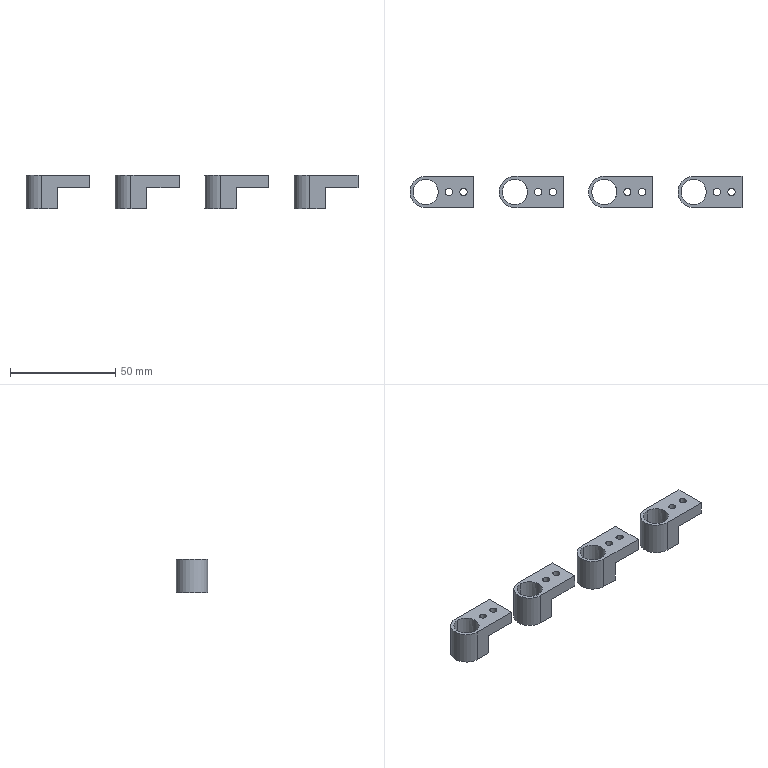Part | 4 solids | 64 faces | box 158 x 15 x 16 mm | volume 10731 mm3 | cylinder 36 | plane 28 | commonest cylinder face diameters 3.4 x16 2.5 x8 12 x8 15 x4